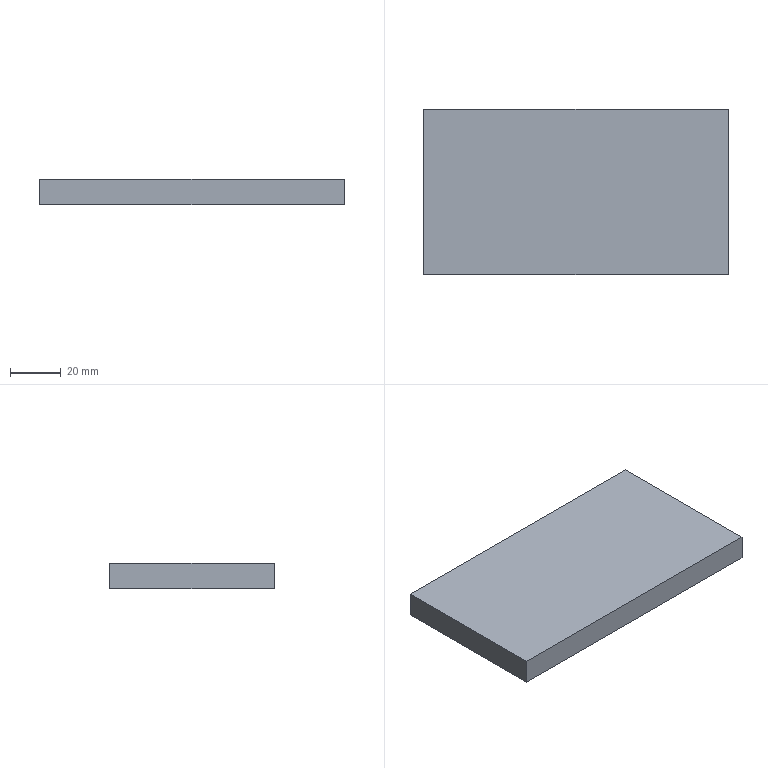Part | NX | features BREP 1 | 1 solid | 6 faces | box 120 x 65 x 10 mm | volume 78000 mm3 | plane 6
STEP:
#1=CARTESIAN_POINT('',(-60.,32.5,-5.));
#2=VERTEX_POINT('',#1);
#3=CARTESIAN_POINT('',(-60.,-32.5,-5.));
#4=VERTEX_POINT('',#3);
#5=CARTESIAN_POINT('',(-60.,32.5,-5.));
#6=DIRECTION('',(0.,-1.,0.));
#7=VECTOR('',#6,1000.);
#8=LINE('',#5,#7);
#9=EDGE_CURVE('',#2,#4,#8,.T.);
#10=ORIENTED_EDGE('',*,*,#9,.T.);
#11=CARTESIAN_POINT('',(-60.,-32.5,5.));
#12=VERTEX_POINT('',#11);
#13=CARTESIAN_POINT('',(-60.,-32.5,5.));
#14=DIRECTION('',(0.,0.,-1.));
#15=VECTOR('',#14,1000.);
#16=LINE('',#13,#15);
#17=EDGE_CURVE('',#12,#4,#16,.T.);
#18=ORIENTED_EDGE('',*,*,#17,.F.);
#19=CARTESIAN_POINT('',(-60.,32.5,5.));
#20=VERTEX_POINT('',#19);
#21=CARTESIAN_POINT('',(-60.,32.5,5.));
#22=DIRECTION('',(0.,-1.,0.));
#23=VECTOR('',#22,1000.);
#24=LINE('',#21,#23);
#25=EDGE_CURVE('',#20,#12,#24,.T.);
#26=ORIENTED_EDGE('',*,*,#25,.F.);
#27=CARTESIAN_POINT('',(-60.,32.5,5.));
#28=DIRECTION('',(0.,0.,-1.));
#29=VECTOR('',#28,1000.);
#30=LINE('',#27,#29);
#31=EDGE_CURVE('',#20,#2,#30,.T.);
#32=ORIENTED_EDGE('',*,*,#31,.T.);
#33=EDGE_LOOP('',(#10,#18,#26,#32));
#34=FACE_BOUND('',#33,.T.);
#35=CARTESIAN_POINT('',(-60.,32.5,5.));
#36=DIRECTION('',(1.,0.,0.));
#37=DIRECTION('',(0.,0.,1.));
#38=AXIS2_PLACEMENT_3D('',#35,#36,#37);
#39=PLANE('',#38);
#40=ADVANCED_FACE('',(#34),#39,.F.);
#41=CARTESIAN_POINT('',(60.,-32.5,-5.));
#42=VERTEX_POINT('',#41);
#43=CARTESIAN_POINT('',(-60.,-32.5,-5.));
#44=DIRECTION('',(1.,0.,0.));
#45=VECTOR('',#44,1000.);
#46=LINE('',#43,#45);
#47=EDGE_CURVE('',#4,#42,#46,.T.);
#48=ORIENTED_EDGE('',*,*,#47,.T.);
#49=CARTESIAN_POINT('',(60.,-32.5,5.));
#50=VERTEX_POINT('',#49);
#51=CARTESIAN_POINT('',(60.,-32.5,5.));
#52=DIRECTION('',(0.,0.,-1.));
#53=VECTOR('',#52,1000.);
#54=LINE('',#51,#53);
#55=EDGE_CURVE('',#50,#42,#54,.T.);
#56=ORIENTED_EDGE('',*,*,#55,.F.);
#57=CARTESIAN_POINT('',(-60.,-32.5,5.));
#58=DIRECTION('',(1.,0.,0.));
#59=VECTOR('',#58,1000.);
#60=LINE('',#57,#59);
#61=EDGE_CURVE('',#12,#50,#60,.T.);
#62=ORIENTED_EDGE('',*,*,#61,.F.);
#63=ORIENTED_EDGE('',*,*,#17,.T.);
#64=EDGE_LOOP('',(#48,#56,#62,#63));
#65=FACE_BOUND('',#64,.T.);
#66=CARTESIAN_POINT('',(-60.,-32.5,5.));
#67=DIRECTION('',(0.,1.,0.));
#68=DIRECTION('',(0.,0.,-1.));
#69=AXIS2_PLACEMENT_3D('',#66,#67,#68);
#70=PLANE('',#69);
#71=ADVANCED_FACE('',(#65),#70,.F.);
#72=CARTESIAN_POINT('',(60.,32.5,-5.));
#73=VERTEX_POINT('',#72);
#74=CARTESIAN_POINT('',(60.,32.5,-5.));
#75=DIRECTION('',(0.,1.,0.));
#76=VECTOR('',#75,1000.);
#77=LINE('',#74,#76);
#78=EDGE_CURVE('',#42,#73,#77,.T.);
#79=ORIENTED_EDGE('',*,*,#78,.T.);
#80=CARTESIAN_POINT('',(60.,32.5,5.));
#81=VERTEX_POINT('',#80);
#82=CARTESIAN_POINT('',(60.,32.5,5.));
#83=DIRECTION('',(0.,0.,-1.));
#84=VECTOR('',#83,1000.);
#85=LINE('',#82,#84);
#86=EDGE_CURVE('',#81,#73,#85,.T.);
#87=ORIENTED_EDGE('',*,*,#86,.F.);
#88=CARTESIAN_POINT('',(60.,32.5,5.));
#89=DIRECTION('',(0.,1.,0.));
#90=VECTOR('',#89,1000.);
#91=LINE('',#88,#90);
#92=EDGE_CURVE('',#50,#81,#91,.T.);
#93=ORIENTED_EDGE('',*,*,#92,.F.);
#94=ORIENTED_EDGE('',*,*,#55,.T.);
#95=EDGE_LOOP('',(#79,#87,#93,#94));
#96=FACE_BOUND('',#95,.T.);
#97=CARTESIAN_POINT('',(60.,32.5,5.));
#98=DIRECTION('',(-1.,0.,0.));
#99=DIRECTION('',(0.,0.,-1.));
#100=AXIS2_PLACEMENT_3D('',#97,#98,#99);
#101=PLANE('',#100);
#102=ADVANCED_FACE('',(#96),#101,.F.);
#103=CARTESIAN_POINT('',(-60.,32.5,-5.));
#104=DIRECTION('',(-1.,0.,0.));
#105=VECTOR('',#104,1000.);
#106=LINE('',#103,#105);
#107=EDGE_CURVE('',#73,#2,#106,.T.);
#108=ORIENTED_EDGE('',*,*,#107,.T.);
#109=ORIENTED_EDGE('',*,*,#31,.F.);
#110=CARTESIAN_POINT('',(-60.,32.5,5.));
#111=DIRECTION('',(-1.,0.,0.));
#112=VECTOR('',#111,1000.);
#113=LINE('',#110,#112);
#114=EDGE_CURVE('',#81,#20,#113,.T.);
#115=ORIENTED_EDGE('',*,*,#114,.F.);
#116=ORIENTED_EDGE('',*,*,#86,.T.);
#117=EDGE_LOOP('',(#108,#109,#115,#116));
#118=FACE_BOUND('',#117,.T.);
#119=CARTESIAN_POINT('',(-60.,32.5,5.));
#120=DIRECTION('',(0.,-1.,0.));
#121=DIRECTION('',(0.,0.,1.));
#122=AXIS2_PLACEMENT_3D('',#119,#120,#121);
#123=PLANE('',#122);
#124=ADVANCED_FACE('',(#118),#123,.F.);
#125=ORIENTED_EDGE('',*,*,#25,.T.);
#126=ORIENTED_EDGE('',*,*,#61,.T.);
#127=ORIENTED_EDGE('',*,*,#92,.T.);
#128=ORIENTED_EDGE('',*,*,#114,.T.);
#129=EDGE_LOOP('',(#125,#126,#127,#128));
#130=FACE_BOUND('',#129,.T.);
#131=CARTESIAN_POINT('',(-60.,-32.5,5.));
#132=DIRECTION('',(0.,0.,1.));
#133=DIRECTION('',(-1.,0.,0.));
#134=AXIS2_PLACEMENT_3D('',#131,#132,#133);
#135=PLANE('',#134);
#136=ADVANCED_FACE('',(#130),#135,.T.);
#137=ORIENTED_EDGE('',*,*,#9,.F.);
#138=ORIENTED_EDGE('',*,*,#107,.F.);
#139=ORIENTED_EDGE('',*,*,#78,.F.);
#140=ORIENTED_EDGE('',*,*,#47,.F.);
#141=EDGE_LOOP('',(#137,#138,#139,#140));
#142=FACE_BOUND('',#141,.T.);
#143=CARTESIAN_POINT('',(-60.,-32.5,-5.));
#144=DIRECTION('',(0.,0.,1.));
#145=DIRECTION('',(-1.,0.,0.));
#146=AXIS2_PLACEMENT_3D('',#143,#144,#145);
#147=PLANE('',#146);
#148=ADVANCED_FACE('',(#142),#147,.F.);
#149=CLOSED_SHELL('',(#40,#71,#102,#124,#136,#148));
#150=MANIFOLD_SOLID_BREP('',#149);
#151=(LENGTH_UNIT()NAMED_UNIT(*)SI_UNIT(.MILLI.,.METRE.));
#152=UNCERTAINTY_MEASURE_WITH_UNIT(LENGTH_MEASURE(0.00001),#151,'','');
#153=(NAMED_UNIT(*)PLANE_ANGLE_UNIT()SI_UNIT($,.RADIAN.));
#154=(NAMED_UNIT(*)SI_UNIT($,.STERADIAN.)SOLID_ANGLE_UNIT());
#155=(GEOMETRIC_REPRESENTATION_CONTEXT(3)GLOBAL_UNCERTAINTY_ASSIGNED_CONTEXT((#152))GLOBAL_UNIT_ASSIGNED_CONTEXT((#151,#153,#154))REPRESENTATION_CONTEXT('',''));
#156=ADVANCED_BREP_SHAPE_REPRESENTATION('',(#150),#155);